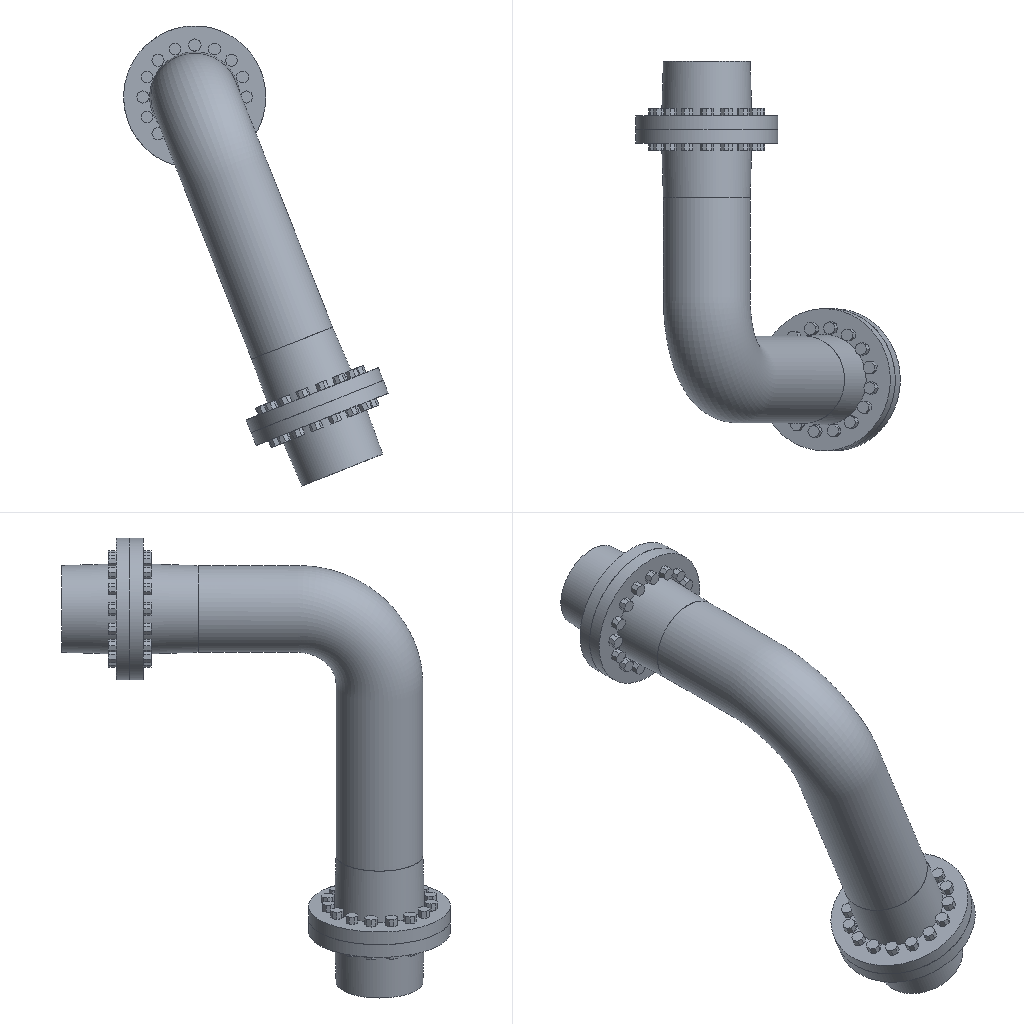Simulation study | abaqus
Set-up summary:
category,name,step,type,value,unit,region
solver,abaqus
solver,version,,,Abaqus/Explicit 2020
units,not stated in the deck,,not stated
analysis,deck,,transient,transient
load_step,Step-1,Step-1,transient
load_step,requested,,,1
mesh,nodes,,,69898
mesh,elements,,,46088
element_type,C3D8R,,solid,46088
load,load commands in deck,,count,4
bc,support commands in deck,,count,1
material,GUAN,,in results
material,SHUAN,,in results
check,setup vs results,,match,"per instance, exact: element labels, types and connectivity; labels of the nodes the elements use; coordinates of those nodes at SINGLE_PRECISION in 36 of 37 instance(s)"
Abaqus input file, long lists of numbers shortened, first 398 of 1239 lines:
*Heading
** Job name: Job-1 Model name: Model-1
** Generated by: Abaqus/CAE 2020
*Preprint, echo=NO, model=NO, history=NO, contact=NO
**
** PARTS
**
*Part, name=work-1
*Node
      1,   7.516,   71.639,    327.175
      2,   28.109,   71.639,   296.355
** (11603 more lines like these left out)
*Element, type=C3D8R
  1, 1914, 1854,  144,  143, 7833, 7773, 2131, 2140
  2, 1913, 1855, 1854, 1914, 7832, 7774, 7773, 7833
** (7830 more lines like these left out)
*Nset, nset=Set-2, generate
     1,  11605,      1
*Elset, elset=Set-2, generate
    1,  7832,     1
** Section: guan
*Solid Section, elset=Set-2, material=guan
,
*End Part
**
*Part, name=work-2
*Node
      1,   -133.467,  -53.341,   303.478
      2,   -129.716,  -53.341,   300.992
** (11398 more lines like these left out)
*Element, type=C3D8R
   1,   121,   122,   133,   162,     1,     2,    13,    42
   2,   162,   133,   134,   161,    42,    13,    14,    41
** (5638 more lines like these left out)
*Nset, nset=Set-2, generate
     1,  11400,      1
*Elset, elset=Set-2, generate
    1,  5640,     1
** Section: guan
*Solid Section, elset=Set-2, material=guan
,
*End Part
**
*Part, name=work-3
*Node
      1,   251.619,  -399.758,   -269.833
      2,   277.179,  -403.562,  -259.721
** (13338 more lines like these left out)
*Element, type=C3D8R
  1, 1985, 1926,  167,  166, 9413, 9354, 2193, 2202
  2, 1984, 1927, 1926, 1985, 9412, 9355, 9354, 9413
** (9574 more lines like these left out)
*Nset, nset=Set-2, generate
     1,  13340,      1
*Elset, elset=Set-2, generate
    1,  9576,     1
** Section: guan
*Solid Section, elset=Set-2, material=guan
,
*End Part
**
*Part, name=work-8
*Node
      1,  -77.419,   46.139,   165.583
      2,  -77.419,   46.139,   158.333
** (267 more lines like these left out)
*Element, type=C3D8R
 1, 130,  31, 123, 229,  29,   1,  30, 122
 2, 131,  32, 124, 228, 130,  31, 123, 229
** (174 more lines like these left out)
*Nset, nset=Set-1, generate
   1,  269,    1
*Elset, elset=Set-1, generate
   1,  176,    1
** Section: shuan
*Solid Section, elset=Set-1, material=shuan
,
*End Part
**
*Part, name=work-39
*Node
      1,    170.135,  -290.816,  -328.954
      2,   170.243,   -283.567,  -328.911
** (267 more lines like these left out)
*Element, type=C3D8R
 1, 130,  37, 123, 229,  29,   1,  30, 122
 2, 131,  36, 124, 228, 130,  37, 123, 229
** (174 more lines like these left out)
*Nset, nset=Set-1, generate
   1,  269,    1
*Elset, elset=Set-1, generate
   1,  176,    1
** Section: shuan
*Solid Section, elset=Set-1, material=shuan
,
*End Part
**
**
** ASSEMBLY
**
*Assembly, name=Assembly
**
*Instance, name=work-1-1, part=work-1
*End Instance
**
*Instance, name=work-2-1, part=work-2
*End Instance
**
*Instance, name=work-3-1, part=work-3
*End Instance
**
*Instance, name=work-8-1, part=work-8
   10.51,     0.5,    -0.5831
*End Instance
**
*Instance, name=work-39-1, part=work-39
   10.692,    -0.1838,     4.23
*End Instance
**
*Instance, name=work-1-2, part=work-1
 -133.819,   143.277,           0.
 -133.819,   143.277,           0.,  -133.819,   143.277,           1.,         180.
*End Instance
**
*Instance, name=work-3-2, part=work-3
156.459, -747.905, -676.855
156.459, -747.905, -676.855, 157.38, -748.043, -676.49,         180.
*End Instance
**
*Instance, name=work-39-1-rad-2, part=work-39
-124.956, -37.925, -49.433
-124.956, -37.925, -49.433, -125.324, -37.925, -48.504, 22.5
*End Instance
**
*Instance, name=work-39-1-rad-3, part=work-39
-236.848, -128.617, -93.699
-236.848, -128.617, -93.699, -237.216, -128.617, -92.769, 45.
*End Instance
**
*Instance, name=work-39-1-rad-4, part=work-39
-307.95, -258.454, -121.827
-307.95, -258.454, -121.827, -308.318, -258.454, -120.898, 67.5
*End Instance
**
*Instance, name=work-39-1-rad-5, part=work-39
-327.438, -407.67, -129.537
-327.438, -407.67, -129.537, -327.806, -407.67, -128.607, 90.
*End Instance
**
*Instance, name=work-39-1-rad-6, part=work-39
-292.343, -553.547, -115.653
-292.343, -553.547, -115.653, -292.711, -553.547, -114.723, 112.5
*End Instance
**
*Instance, name=work-39-1-rad-7, part=work-39
-208.01, -673.877, -82.29
-208.01, -673.877, -82.29, -208.378, -673.877, -81.361, 135.
*End Instance
**
*Instance, name=work-39-1-rad-8, part=work-39
-87.277, -750.341, -34.528
-87.277, -750.341, -34.528, -87.645, -750.341, -33.598, 157.5
*End Instance
**
*Instance, name=work-39-1-rad-9, part=work-39
51.475,  -771.298, 20.364
51.475,  -771.298, 20.364, 51.107,  -771.298, 21.294,         180.
*End Instance
**
*Instance, name=work-39-1-rad-10, part=work-39
187.123, -733.558, 74.027
187.123, -733.558, 74.027, 186.755, -733.558, 74.957, 202.5
*End Instance
**
*Instance, name=work-39-1-rad-11, part=work-39
299.015, -642.865, 118.293
299.015, -642.865, 118.293, 298.647, -642.865, 119.223, 225.
*End Instance
**
*Instance, name=work-39-1-rad-12, part=work-39
370.118, -513.028, 146.421
370.118, -513.028, 146.421, 370.485, -513.028, 145.491, 112.5
*End Instance
**
*Instance, name=work-39-1-rad-13, part=work-39
389.605, -363.812, 154.131
389.605, -363.812, 154.131, 389.973, -363.812, 153.201, 90.
*End Instance
**
*Instance, name=work-39-1-rad-14, part=work-39
354.511, -217.935, 140.247
354.511, -217.935, 140.247, 354.879, -217.935, 139.317, 67.5
*End Instance
**
*Instance, name=work-39-1-rad-15, part=work-39
270.178, -97.605, 106.884
270.178, -97.605, 106.884, 270.545, -97.605, 105.954, 45.
*End Instance
**
*Instance, name=work-39-1-rad-16, part=work-39
149.445, -21.141, 59.121
149.445, -21.141, 59.121, 149.812, -21.141, 58.192, 22.5
*End Instance
**
*Instance, name=work-8-1-rad-2, part=work-8
104.338,     0.5, 48.88
104.338,     0.5, 48.88, 104.338, -0.5, 48.88, 22.5
*End Instance
**
*Instance, name=work-8-1-rad-3, part=work-8
172.094,     0.5, 130.484
172.094,     0.5, 130.484, 172.094, -0.5, 130.484, 45.
*End Instance
**
*Instance, name=work-8-1-rad-4, part=work-8
203.465,     0.5, 231.805
203.465,     0.5, 231.805, 203.465, -0.5, 231.805, 67.5
*End Instance
**
*Instance, name=work-8-1-rad-5, part=work-8
  193.674,     0.5,   337.419
  193.674,     0.5,   337.419,   193.674, -0.5,   337.419, 90.
*End Instance
**
*Instance, name=work-8-1-rad-6, part=work-8
144.211,     0.5, 431.247
144.211,     0.5, 431.247, 144.211, -0.5, 431.247, 112.5
*End Instance
**
*Instance, name=work-8-1-rad-7, part=work-8
62.607,     0.5, 499.004
62.607,     0.5, 499.004, 62.607, 1.5, 499.004, 225.
*End Instance
**
*Instance, name=work-8-1-rad-8, part=work-8
-38.715,     0.5, 530.374
-38.715,     0.5, 530.374, -38.715, 1.5, 530.374, 202.5
*End Instance
**
*Instance, name=work-8-1-rad-9, part=work-8
 -144.329,     0.5,   520.583
 -144.329,     0.5,   520.583,  -144.329,     1.5,   520.583,         180.
*End Instance
**
*Instance, name=work-8-1-rad-10, part=work-8
-238.156,     0.5, 471.12
-238.156,     0.5, 471.12, -238.156, 1.5, 471.12, 157.5
*End Instance
**
*Instance, name=work-8-1-rad-11, part=work-8
-305.913,     0.5, 389.516
-305.913,     0.5, 389.516, -305.913, 1.5, 389.516, 135.
*End Instance
**
*Instance, name=work-8-1-rad-12, part=work-8
-337.284,     0.5, 288.195
-337.284,     0.5, 288.195, -337.284, 1.5, 288.195, 112.5
*End Instance
**
*Instance, name=work-8-1-rad-13, part=work-8
 -327.493,     0.5,   182.581
 -327.493,     0.5,   182.581,  -327.493, 1.5,   182.581, 90.
*End Instance
**
*Instance, name=work-8-1-rad-14, part=work-8
-278.03,     0.5, 88.753
-278.03,     0.5, 88.753, -278.03, 1.5, 88.753, 67.5
*End Instance
**
*Instance, name=work-8-1-rad-15, part=work-8
-196.426,     0.5, 20.996
-196.426,     0.5, 20.996, -196.426, 1.5, 20.996, 45.
*End Instance
**
*Instance, name=work-8-1-rad-16, part=work-8
-95.104,     0.5, -10.374
-95.104,     0.5, -10.374, -95.104, 1.5, -10.374, 22.5
*End Instance
**
*Nset, nset=Set-1, instance=work-1-1, generate
     1,  11605,      1
*Nset, nset=Set-1, instance=work-2-1, generate
     1,  11400,      1
*Nset, nset=Set-1, instance=work-3-1, generate
     1,  13340,      1
*Nset, nset=Set-1, instance=work-39-1-rad-2, generate
   1,  269,    1
*Nset, nset=Set-1, instance=work-39-1-rad-10, generate
   1,  269,    1
*Nset, nset=Set-1, instance=work-39-1-rad-6, generate
   1,  269,    1
*Nset, nset=Set-1, instance=work-39-1-rad-14, generate
   1,  269,    1
*Nset, nset=Set-1, instance=work-1-2, generate
     1,  11605,      1
*Nset, nset=Set-1, instance=work-39-1-rad-4, generate
   1,  269,    1
*Nset, nset=Set-1, instance=work-39-1-rad-12, generate
   1,  269,    1
*Nset, nset=Set-1, instance=work-39-1-rad-8, generate
   1,  269,    1
*Nset, nset=Set-1, instance=work-39-1-rad-16, generate
   1,  269,    1
*Nset, nset=Set-1, instance=work-8-1, generate
   1,  269,    1
*Nset, nset=Set-1, instance=work-39-1, generate
   1,  269,    1
*Nset, nset=Set-1, instance=work-39-1-rad-3, generate
   1,  269,    1
*Nset, nset=Set-1, instance=work-39-1-rad-11, generate
   1,  269,    1
*Nset, nset=Set-1, instance=work-3-2, generate
     1,  13340,      1
*Nset, nset=Set-1, instance=work-39-1-rad-7, generate
   1,  269,    1
*Nset, nset=Set-1, instance=work-39-1-rad-15, generate
   1,  269,    1
*Nset, nset=Set-1, instance=work-39-1-rad-5, generate
   1,  269,    1
*Nset, nset=Set-1, instance=work-39-1-rad-13, generate
   1,  269,    1
*Nset, nset=Set-1, instance=work-39-1-rad-9, generate
   1,  269,    1
*Nset, nset=Set-1, instance=work-8-1-rad-2, generate
   1,  269,    1
*Nset, nset=Set-1, instance=work-8-1-rad-4, generate
   1,  269,    1
*Nset, nset=Set-1, instance=work-8-1-rad-6, generate
   1,  269,    1
*Nset, nset=Set-1, instance=work-8-1-rad-10, generate
   1,  269,    1
*Nset, nset=Set-1, instance=work-8-1-rad-14, generate
   1,  269,    1
*Nset, nset=Set-1, instance=work-8-1-rad-8, generate
   1,  269,    1
*Nset, nset=Set-1, instance=work-8-1-rad-12, generate
   1,  269,    1
*Nset, nset=Set-1, instance=work-8-1-rad-16, generate
   1,  269,    1
*Nset, nset=Set-1, instance=work-8-1-rad-3, generate
   1,  269,    1
*Nset, nset=Set-1, instance=work-8-1-rad-7, generate
   1,  269,    1
*Nset, nset=Set-1, instance=work-8-1-rad-11, generate
   1,  269,    1
*Nset, nset=Set-1, instance=work-8-1-rad-15, generate
   1,  269,    1
*Nset, nset=Set-1, instance=work-8-1-rad-5, generate
   1,  269,    1
*Nset, nset=Set-1, instance=work-8-1-rad-13, generate
   1,  269,    1
*Nset, nset=Set-1, instance=work-8-1-rad-9, generate
   1,  269,    1
*Elset, elset=Set-1, instance=work-1-1, generate
    1,  7832,     1
*Elset, elset=Set-1, instance=work-2-1, generate
    1,  5640,     1
*Elset, elset=Set-1, instance=work-3-1, generate
    1,  9576,     1
*Elset, elset=Set-1, instance=work-39-1-rad-2, generate
   1,  176,    1
*Elset, elset=Set-1, instance=work-39-1-rad-10, generate
   1,  176,    1
*Elset, elset=Set-1, instance=work-39-1-rad-6, generate
   1,  176,    1
*Elset, elset=Set-1, instance=work-39-1-rad-14, generate
   1,  176,    1
*Elset, elset=Set-1, instance=work-1-2, generate
    1,  7832,     1
*Elset, elset=Set-1, instance=work-39-1-rad-4, generate
   1,  176,    1
*Elset, elset=Set-1, instance=work-39-1-rad-12, generate
   1,  176,    1
*Elset, elset=Set-1, instance=work-39-1-rad-8, generate
   1,  176,    1
*Elset, elset=Set-1, instance=work-39-1-rad-16, generate
   1,  176,    1
*Elset, elset=Set-1, instance=work-8-1, generate
   1,  176,    1
*Elset, elset=Set-1, instance=work-39-1, generate
   1,  176,    1
*Elset, elset=Set-1, instance=work-39-1-rad-3, generate
   1,  176,    1
*Elset, elset=Set-1, instance=work-39-1-rad-11, generate
   1,  176,    1
*Elset, elset=Set-1, instance=work-3-2, generate
    1,  9576,     1
*Elset, elset=Set-1, instance=work-39-1-rad-7, generate
   1,  176,    1
*Elset, elset=Set-1, instance=work-39-1-rad-15, generate
   1,  176,    1
*Elset, elset=Set-1, instance=work-39-1-rad-5, generate
   1,  176,    1
*Elset, elset=Set-1, instance=work-39-1-rad-13, generate
   1,  176,    1
*Elset, elset=Set-1, instance=work-39-1-rad-9, generate
   1,  176,    1
*Elset, elset=Set-1, instance=work-8-1-rad-2, generate
Last 584 lines:
** (233 more lines like these left out)
*Elset, elset=_Surf-17_S5, internal, instance=work-3-1, generate
 7729,  9576,     1
*Surface, type=ELEMENT, name=Surf-17
_Surf-17_S3, S3
_Surf-17_S6, S6
_Surf-17_S4, S4
_Surf-17_S5, S5
*Elset, elset=_Surf-18_S4, internal, instance=work-2-1
    1,    2,    3,    4,    5,    6,    7,    8,    9,   10,   11,   12,   13,   14,   15,   16
   23,   24,   25,   26,   27,   28,   29,   30,   31,   32,   33,   34,   35,   36,   37,   38
** (233 more lines like these left out)
*Elset, elset=_Surf-18_S6, internal, instance=work-2-1
   17,   18,   19,   20,   21,   22,   47,   48,   49,   50,   51,   52,   53,   54,   55,   56
   57,   58,   59,   60,   77,   78,   79,   80,   81,   82,  107,  108,  109,  110,  111,  112
** (116 more lines like these left out)
*Surface, type=ELEMENT, name=Surf-18
_Surf-18_S4, S4
_Surf-18_S6, S6
*Elset, elset=_m_Surf-5_S4, internal, instance=work-1-1
 4244, 4264, 4285, 4305, 4326, 4346, 4367, 4387, 4408, 4428, 4449, 4469, 4490, 4510, 4531, 4551
 4572, 4592, 4613, 4633, 4654, 4674, 4695, 4715, 4736, 4756, 4777, 4797, 4818, 4838, 4859, 4879
** (9 more lines like these left out)
*Elset, elset=_m_Surf-5_S4, internal, instance=work-3-1, generate
 7749,  9576,    21
*Surface, type=ELEMENT, name=m_Surf-5
_m_Surf-5_S4, S4
*Elset, elset=_m_Surf-7_S1, internal, instance=work-1-2
    1,    2,    3,    4,    5,    6,    7,    8,    9,   10,   11,   12,   13,   14,   15,   16
   17,   18,   19,   20,   21,   22,   23,   24,   25,   26,   27,   28,   29,   30,   31,   32
** (60 more lines like these left out)
*Surface, type=ELEMENT, name=m_Surf-7
_m_Surf-7_S1, S1
*Elset, elset=_m_Surf-9_S5, internal, instance=work-1-2, generate
 4265,  7832,    41
*Elset, elset=_m_Surf-9_S1, internal, instance=work-1-2
    1,    2,    3,    4,    5,    6,    7,    8,    9,   10,   11,   12,   13,   14,   15,   16
   17,   18,   19,   20,   21,   22,   23,   24,   25,   26,   27,   28,   29,   30,   31,   32
** (60 more lines like these left out)
*Surface, type=ELEMENT, name=m_Surf-9
_m_Surf-9_S5, S5
_m_Surf-9_S1, S1
*Elset, elset=_m_Surf-10_S3, internal, instance=work-3-2, generate
 2999,  6740,    43
*Elset, elset=_m_Surf-10_S6, internal, instance=work-3-2, generate
 7729,  9556,    21
*Elset, elset=_m_Surf-10_S1, internal, instance=work-3-2
    1,    2,    3,    4,    5,    6,    7,    8,    9,   10,   11,   12,   13,   14,   15,   16
   17,   18,   19,   20,   21,   22,   23,   24,   25,   26,   27,   28,   29,   30,   31,   32
** (60 more lines like these left out)
*Surface, type=ELEMENT, name=m_Surf-10
_m_Surf-10_S3, S3
_m_Surf-10_S6, S6
_m_Surf-10_S1, S1
*Elset, elset=_m_Surf-12_S5, internal, instance=work-1-2, generate
 4265,  7832,    41
*Elset, elset=_m_Surf-12_S1, internal, instance=work-1-2
    1,    2,    3,    4,    5,    6,    7,    8,    9,   10,   11,   12,   13,   14,   15,   16
   17,   18,   19,   20,   21,   22,   23,   24,   25,   26,   27,   28,   29,   30,   31,   32
** (60 more lines like these left out)
*Surface, type=ELEMENT, name=m_Surf-12
_m_Surf-12_S5, S5
_m_Surf-12_S1, S1
*Elset, elset=_m_Surf-13_S1, internal, instance=work-8-1
  97,  98, 107, 108, 117, 118, 130, 131, 137, 138, 147, 148, 157, 158, 167, 168
*Elset, elset=_m_Surf-13_S1, internal, instance=work-8-1-rad-2
  97,  98, 107, 108, 117, 118, 130, 131, 137, 138, 147, 148, 157, 158, 167, 168
*Elset, elset=_m_Surf-13_S1, internal, instance=work-8-1-rad-4
  97,  98, 107, 108, 117, 118, 130, 131, 137, 138, 147, 148, 157, 158, 167, 168
*Elset, elset=_m_Surf-13_S1, internal, instance=work-8-1-rad-6
  97,  98, 107, 108, 117, 118, 130, 131, 137, 138, 147, 148, 157, 158, 167, 168
*Elset, elset=_m_Surf-13_S1, internal, instance=work-8-1-rad-10
  97,  98, 107, 108, 117, 118, 130, 131, 137, 138, 147, 148, 157, 158, 167, 168
*Elset, elset=_m_Surf-13_S1, internal, instance=work-8-1-rad-14
  97,  98, 107, 108, 117, 118, 130, 131, 137, 138, 147, 148, 157, 158, 167, 168
*Elset, elset=_m_Surf-13_S1, internal, instance=work-8-1-rad-8
  97,  98, 107, 108, 117, 118, 130, 131, 137, 138, 147, 148, 157, 158, 167, 168
*Elset, elset=_m_Surf-13_S1, internal, instance=work-8-1-rad-12
  97,  98, 107, 108, 117, 118, 130, 131, 137, 138, 147, 148, 157, 158, 167, 168
*Elset, elset=_m_Surf-13_S1, internal, instance=work-8-1-rad-16
  97,  98, 107, 108, 117, 118, 130, 131, 137, 138, 147, 148, 157, 158, 167, 168
*Elset, elset=_m_Surf-13_S1, internal, instance=work-8-1-rad-3
  97,  98, 107, 108, 117, 118, 130, 131, 137, 138, 147, 148, 157, 158, 167, 168
*Elset, elset=_m_Surf-13_S1, internal, instance=work-8-1-rad-7
  97,  98, 107, 108, 117, 118, 130, 131, 137, 138, 147, 148, 157, 158, 167, 168
*Elset, elset=_m_Surf-13_S1, internal, instance=work-8-1-rad-11
  97,  98, 107, 108, 117, 118, 130, 131, 137, 138, 147, 148, 157, 158, 167, 168
*Elset, elset=_m_Surf-13_S1, internal, instance=work-8-1-rad-15
  97,  98, 107, 108, 117, 118, 130, 131, 137, 138, 147, 148, 157, 158, 167, 168
*Elset, elset=_m_Surf-13_S1, internal, instance=work-8-1-rad-5
  97,  98, 107, 108, 117, 118, 130, 131, 137, 138, 147, 148, 157, 158, 167, 168
*Elset, elset=_m_Surf-13_S1, internal, instance=work-8-1-rad-13
  97,  98, 107, 108, 117, 118, 130, 131, 137, 138, 147, 148, 157, 158, 167, 168
*Elset, elset=_m_Surf-13_S1, internal, instance=work-8-1-rad-9
  97,  98, 107, 108, 117, 118, 130, 131, 137, 138, 147, 148, 157, 158, 167, 168
*Elset, elset=_m_Surf-13_S3, internal, instance=work-8-1
  5,  6,  7,  8, 17, 18, 19, 20, 25, 26, 27, 28, 49, 50, 51, 52
 73, 74, 75, 76, 89, 90, 91, 92, 93, 94, 95, 96
*Elset, elset=_m_Surf-13_S3, internal, instance=work-8-1-rad-2
  5,  6,  7,  8, 17, 18, 19, 20, 25, 26, 27, 28, 49, 50, 51, 52
 73, 74, 75, 76, 89, 90, 91, 92, 93, 94, 95, 96
*Elset, elset=_m_Surf-13_S3, internal, instance=work-8-1-rad-4
  5,  6,  7,  8, 17, 18, 19, 20, 25, 26, 27, 28, 49, 50, 51, 52
 73, 74, 75, 76, 89, 90, 91, 92, 93, 94, 95, 96
*Elset, elset=_m_Surf-13_S3, internal, instance=work-8-1-rad-6
  5,  6,  7,  8, 17, 18, 19, 20, 25, 26, 27, 28, 49, 50, 51, 52
 73, 74, 75, 76, 89, 90, 91, 92, 93, 94, 95, 96
*Elset, elset=_m_Surf-13_S3, internal, instance=work-8-1-rad-10
  5,  6,  7,  8, 17, 18, 19, 20, 25, 26, 27, 28, 49, 50, 51, 52
 73, 74, 75, 76, 89, 90, 91, 92, 93, 94, 95, 96
*Elset, elset=_m_Surf-13_S3, internal, instance=work-8-1-rad-14
  5,  6,  7,  8, 17, 18, 19, 20, 25, 26, 27, 28, 49, 50, 51, 52
 73, 74, 75, 76, 89, 90, 91, 92, 93, 94, 95, 96
*Elset, elset=_m_Surf-13_S3, internal, instance=work-8-1-rad-8
  5,  6,  7,  8, 17, 18, 19, 20, 25, 26, 27, 28, 49, 50, 51, 52
 73, 74, 75, 76, 89, 90, 91, 92, 93, 94, 95, 96
*Elset, elset=_m_Surf-13_S3, internal, instance=work-8-1-rad-12
  5,  6,  7,  8, 17, 18, 19, 20, 25, 26, 27, 28, 49, 50, 51, 52
 73, 74, 75, 76, 89, 90, 91, 92, 93, 94, 95, 96
*Elset, elset=_m_Surf-13_S3, internal, instance=work-8-1-rad-16
  5,  6,  7,  8, 17, 18, 19, 20, 25, 26, 27, 28, 49, 50, 51, 52
 73, 74, 75, 76, 89, 90, 91, 92, 93, 94, 95, 96
*Elset, elset=_m_Surf-13_S3, internal, instance=work-8-1-rad-3
  5,  6,  7,  8, 17, 18, 19, 20, 25, 26, 27, 28, 49, 50, 51, 52
 73, 74, 75, 76, 89, 90, 91, 92, 93, 94, 95, 96
*Elset, elset=_m_Surf-13_S3, internal, instance=work-8-1-rad-7
  5,  6,  7,  8, 17, 18, 19, 20, 25, 26, 27, 28, 49, 50, 51, 52
 73, 74, 75, 76, 89, 90, 91, 92, 93, 94, 95, 96
*Elset, elset=_m_Surf-13_S3, internal, instance=work-8-1-rad-11
  5,  6,  7,  8, 17, 18, 19, 20, 25, 26, 27, 28, 49, 50, 51, 52
 73, 74, 75, 76, 89, 90, 91, 92, 93, 94, 95, 96
*Elset, elset=_m_Surf-13_S3, internal, instance=work-8-1-rad-15
  5,  6,  7,  8, 17, 18, 19, 20, 25, 26, 27, 28, 49, 50, 51, 52
 73, 74, 75, 76, 89, 90, 91, 92, 93, 94, 95, 96
*Elset, elset=_m_Surf-13_S3, internal, instance=work-8-1-rad-5
  5,  6,  7,  8, 17, 18, 19, 20, 25, 26, 27, 28, 49, 50, 51, 52
 73, 74, 75, 76, 89, 90, 91, 92, 93, 94, 95, 96
*Elset, elset=_m_Surf-13_S3, internal, instance=work-8-1-rad-13
  5,  6,  7,  8, 17, 18, 19, 20, 25, 26, 27, 28, 49, 50, 51, 52
 73, 74, 75, 76, 89, 90, 91, 92, 93, 94, 95, 96
*Elset, elset=_m_Surf-13_S3, internal, instance=work-8-1-rad-9
  5,  6,  7,  8, 17, 18, 19, 20, 25, 26, 27, 28, 49, 50, 51, 52
 73, 74, 75, 76, 89, 90, 91, 92, 93, 94, 95, 96
*Elset, elset=_m_Surf-13_S4, internal, instance=work-8-1
  9, 10, 11, 12, 21, 22, 23, 24, 29, 30, 31, 32, 53, 54, 55, 56
 81, 82, 83, 84
*Elset, elset=_m_Surf-13_S4, internal, instance=work-8-1-rad-2
  9, 10, 11, 12, 21, 22, 23, 24, 29, 30, 31, 32, 53, 54, 55, 56
 81, 82, 83, 84
*Elset, elset=_m_Surf-13_S4, internal, instance=work-8-1-rad-4
  9, 10, 11, 12, 21, 22, 23, 24, 29, 30, 31, 32, 53, 54, 55, 56
 81, 82, 83, 84
*Elset, elset=_m_Surf-13_S4, internal, instance=work-8-1-rad-6
  9, 10, 11, 12, 21, 22, 23, 24, 29, 30, 31, 32, 53, 54, 55, 56
 81, 82, 83, 84
*Elset, elset=_m_Surf-13_S4, internal, instance=work-8-1-rad-10
  9, 10, 11, 12, 21, 22, 23, 24, 29, 30, 31, 32, 53, 54, 55, 56
 81, 82, 83, 84
*Elset, elset=_m_Surf-13_S4, internal, instance=work-8-1-rad-14
  9, 10, 11, 12, 21, 22, 23, 24, 29, 30, 31, 32, 53, 54, 55, 56
 81, 82, 83, 84
*Elset, elset=_m_Surf-13_S4, internal, instance=work-8-1-rad-8
  9, 10, 11, 12, 21, 22, 23, 24, 29, 30, 31, 32, 53, 54, 55, 56
 81, 82, 83, 84
*Elset, elset=_m_Surf-13_S4, internal, instance=work-8-1-rad-12
  9, 10, 11, 12, 21, 22, 23, 24, 29, 30, 31, 32, 53, 54, 55, 56
 81, 82, 83, 84
*Elset, elset=_m_Surf-13_S4, internal, instance=work-8-1-rad-16
  9, 10, 11, 12, 21, 22, 23, 24, 29, 30, 31, 32, 53, 54, 55, 56
 81, 82, 83, 84
*Elset, elset=_m_Surf-13_S4, internal, instance=work-8-1-rad-3
  9, 10, 11, 12, 21, 22, 23, 24, 29, 30, 31, 32, 53, 54, 55, 56
 81, 82, 83, 84
*Elset, elset=_m_Surf-13_S4, internal, instance=work-8-1-rad-7
  9, 10, 11, 12, 21, 22, 23, 24, 29, 30, 31, 32, 53, 54, 55, 56
 81, 82, 83, 84
*Elset, elset=_m_Surf-13_S4, internal, instance=work-8-1-rad-11
  9, 10, 11, 12, 21, 22, 23, 24, 29, 30, 31, 32, 53, 54, 55, 56
 81, 82, 83, 84
*Elset, elset=_m_Surf-13_S4, internal, instance=work-8-1-rad-15
  9, 10, 11, 12, 21, 22, 23, 24, 29, 30, 31, 32, 53, 54, 55, 56
 81, 82, 83, 84
*Elset, elset=_m_Surf-13_S4, internal, instance=work-8-1-rad-5
  9, 10, 11, 12, 21, 22, 23, 24, 29, 30, 31, 32, 53, 54, 55, 56
 81, 82, 83, 84
*Elset, elset=_m_Surf-13_S4, internal, instance=work-8-1-rad-13
  9, 10, 11, 12, 21, 22, 23, 24, 29, 30, 31, 32, 53, 54, 55, 56
 81, 82, 83, 84
*Elset, elset=_m_Surf-13_S4, internal, instance=work-8-1-rad-9
  9, 10, 11, 12, 21, 22, 23, 24, 29, 30, 31, 32, 53, 54, 55, 56
 81, 82, 83, 84
*Elset, elset=_m_Surf-13_S2, internal, instance=work-8-1
 37, 38, 39, 40, 41, 42, 43, 44, 61, 62, 63, 64, 65, 66, 67, 68
*Elset, elset=_m_Surf-13_S2, internal, instance=work-8-1-rad-2
 37, 38, 39, 40, 41, 42, 43, 44, 61, 62, 63, 64, 65, 66, 67, 68
*Elset, elset=_m_Surf-13_S2, internal, instance=work-8-1-rad-4
 37, 38, 39, 40, 41, 42, 43, 44, 61, 62, 63, 64, 65, 66, 67, 68
*Elset, elset=_m_Surf-13_S2, internal, instance=work-8-1-rad-6
 37, 38, 39, 40, 41, 42, 43, 44, 61, 62, 63, 64, 65, 66, 67, 68
*Elset, elset=_m_Surf-13_S2, internal, instance=work-8-1-rad-10
 37, 38, 39, 40, 41, 42, 43, 44, 61, 62, 63, 64, 65, 66, 67, 68
*Elset, elset=_m_Surf-13_S2, internal, instance=work-8-1-rad-14
 37, 38, 39, 40, 41, 42, 43, 44, 61, 62, 63, 64, 65, 66, 67, 68
*Elset, elset=_m_Surf-13_S2, internal, instance=work-8-1-rad-8
 37, 38, 39, 40, 41, 42, 43, 44, 61, 62, 63, 64, 65, 66, 67, 68
*Elset, elset=_m_Surf-13_S2, internal, instance=work-8-1-rad-12
 37, 38, 39, 40, 41, 42, 43, 44, 61, 62, 63, 64, 65, 66, 67, 68
*Elset, elset=_m_Surf-13_S2, internal, instance=work-8-1-rad-16
 37, 38, 39, 40, 41, 42, 43, 44, 61, 62, 63, 64, 65, 66, 67, 68
*Elset, elset=_m_Surf-13_S2, internal, instance=work-8-1-rad-3
 37, 38, 39, 40, 41, 42, 43, 44, 61, 62, 63, 64, 65, 66, 67, 68
*Elset, elset=_m_Surf-13_S2, internal, instance=work-8-1-rad-7
 37, 38, 39, 40, 41, 42, 43, 44, 61, 62, 63, 64, 65, 66, 67, 68
*Elset, elset=_m_Surf-13_S2, internal, instance=work-8-1-rad-11
 37, 38, 39, 40, 41, 42, 43, 44, 61, 62, 63, 64, 65, 66, 67, 68
*Elset, elset=_m_Surf-13_S2, internal, instance=work-8-1-rad-15
 37, 38, 39, 40, 41, 42, 43, 44, 61, 62, 63, 64, 65, 66, 67, 68
*Elset, elset=_m_Surf-13_S2, internal, instance=work-8-1-rad-5
 37, 38, 39, 40, 41, 42, 43, 44, 61, 62, 63, 64, 65, 66, 67, 68
*Elset, elset=_m_Surf-13_S2, internal, instance=work-8-1-rad-13
 37, 38, 39, 40, 41, 42, 43, 44, 61, 62, 63, 64, 65, 66, 67, 68
*Elset, elset=_m_Surf-13_S2, internal, instance=work-8-1-rad-9
 37, 38, 39, 40, 41, 42, 43, 44, 61, 62, 63, 64, 65, 66, 67, 68
*Surface, type=ELEMENT, name=m_Surf-13
_m_Surf-13_S1, S1
_m_Surf-13_S3, S3
_m_Surf-13_S4, S4
_m_Surf-13_S2, S2
*Elset, elset=_m_Surf-15_S1, internal, instance=work-39-1
  97,  98, 107, 108, 117, 118, 127, 128, 140, 141, 147, 148, 160, 161, 167, 168
*Elset, elset=_m_Surf-15_S1, internal, instance=work-39-1-rad-2
  97,  98, 107, 108, 117, 118, 127, 128, 140, 141, 147, 148, 160, 161, 167, 168
*Elset, elset=_m_Surf-15_S1, internal, instance=work-39-1-rad-4
  97,  98, 107, 108, 117, 118, 127, 128, 140, 141, 147, 148, 160, 161, 167, 168
*Elset, elset=_m_Surf-15_S1, internal, instance=work-39-1-rad-6
  97,  98, 107, 108, 117, 118, 127, 128, 140, 141, 147, 148, 160, 161, 167, 168
*Elset, elset=_m_Surf-15_S1, internal, instance=work-39-1-rad-10
  97,  98, 107, 108, 117, 118, 127, 128, 140, 141, 147, 148, 160, 161, 167, 168
*Elset, elset=_m_Surf-15_S1, internal, instance=work-39-1-rad-14
  97,  98, 107, 108, 117, 118, 127, 128, 140, 141, 147, 148, 160, 161, 167, 168
*Elset, elset=_m_Surf-15_S1, internal, instance=work-39-1-rad-8
  97,  98, 107, 108, 117, 118, 127, 128, 140, 141, 147, 148, 160, 161, 167, 168
*Elset, elset=_m_Surf-15_S1, internal, instance=work-39-1-rad-12
  97,  98, 107, 108, 117, 118, 127, 128, 140, 141, 147, 148, 160, 161, 167, 168
*Elset, elset=_m_Surf-15_S1, internal, instance=work-39-1-rad-16
  97,  98, 107, 108, 117, 118, 127, 128, 140, 141, 147, 148, 160, 161, 167, 168
*Elset, elset=_m_Surf-15_S1, internal, instance=work-39-1-rad-3
  97,  98, 107, 108, 117, 118, 127, 128, 140, 141, 147, 148, 160, 161, 167, 168
*Elset, elset=_m_Surf-15_S1, internal, instance=work-39-1-rad-7
  97,  98, 107, 108, 117, 118, 127, 128, 140, 141, 147, 148, 160, 161, 167, 168
*Elset, elset=_m_Surf-15_S1, internal, instance=work-39-1-rad-11
  97,  98, 107, 108, 117, 118, 127, 128, 140, 141, 147, 148, 160, 161, 167, 168
*Elset, elset=_m_Surf-15_S1, internal, instance=work-39-1-rad-15
  97,  98, 107, 108, 117, 118, 127, 128, 140, 141, 147, 148, 160, 161, 167, 168
*Elset, elset=_m_Surf-15_S1, internal, instance=work-39-1-rad-5
  97,  98, 107, 108, 117, 118, 127, 128, 140, 141, 147, 148, 160, 161, 167, 168
*Elset, elset=_m_Surf-15_S1, internal, instance=work-39-1-rad-13
  97,  98, 107, 108, 117, 118, 127, 128, 140, 141, 147, 148, 160, 161, 167, 168
*Elset, elset=_m_Surf-15_S1, internal, instance=work-39-1-rad-9
  97,  98, 107, 108, 117, 118, 127, 128, 140, 141, 147, 148, 160, 161, 167, 168
*Elset, elset=_m_Surf-15_S3, internal, instance=work-39-1
  5,  6,  7,  8, 17, 18, 19, 20, 25, 26, 27, 28, 49, 50, 51, 52
 77, 78, 79, 80, 89, 90, 91, 92, 93, 94, 95, 96
*Elset, elset=_m_Surf-15_S3, internal, instance=work-39-1-rad-2
  5,  6,  7,  8, 17, 18, 19, 20, 25, 26, 27, 28, 49, 50, 51, 52
 77, 78, 79, 80, 89, 90, 91, 92, 93, 94, 95, 96
*Elset, elset=_m_Surf-15_S3, internal, instance=work-39-1-rad-4
  5,  6,  7,  8, 17, 18, 19, 20, 25, 26, 27, 28, 49, 50, 51, 52
 77, 78, 79, 80, 89, 90, 91, 92, 93, 94, 95, 96
*Elset, elset=_m_Surf-15_S3, internal, instance=work-39-1-rad-6
  5,  6,  7,  8, 17, 18, 19, 20, 25, 26, 27, 28, 49, 50, 51, 52
 77, 78, 79, 80, 89, 90, 91, 92, 93, 94, 95, 96
*Elset, elset=_m_Surf-15_S3, internal, instance=work-39-1-rad-10
  5,  6,  7,  8, 17, 18, 19, 20, 25, 26, 27, 28, 49, 50, 51, 52
 77, 78, 79, 80, 89, 90, 91, 92, 93, 94, 95, 96
*Elset, elset=_m_Surf-15_S3, internal, instance=work-39-1-rad-14
  5,  6,  7,  8, 17, 18, 19, 20, 25, 26, 27, 28, 49, 50, 51, 52
 77, 78, 79, 80, 89, 90, 91, 92, 93, 94, 95, 96
*Elset, elset=_m_Surf-15_S3, internal, instance=work-39-1-rad-8
  5,  6,  7,  8, 17, 18, 19, 20, 25, 26, 27, 28, 49, 50, 51, 52
 77, 78, 79, 80, 89, 90, 91, 92, 93, 94, 95, 96
*Elset, elset=_m_Surf-15_S3, internal, instance=work-39-1-rad-12
  5,  6,  7,  8, 17, 18, 19, 20, 25, 26, 27, 28, 49, 50, 51, 52
 77, 78, 79, 80, 89, 90, 91, 92, 93, 94, 95, 96
*Elset, elset=_m_Surf-15_S3, internal, instance=work-39-1-rad-16
  5,  6,  7,  8, 17, 18, 19, 20, 25, 26, 27, 28, 49, 50, 51, 52
 77, 78, 79, 80, 89, 90, 91, 92, 93, 94, 95, 96
*Elset, elset=_m_Surf-15_S3, internal, instance=work-39-1-rad-3
  5,  6,  7,  8, 17, 18, 19, 20, 25, 26, 27, 28, 49, 50, 51, 52
 77, 78, 79, 80, 89, 90, 91, 92, 93, 94, 95, 96
*Elset, elset=_m_Surf-15_S3, internal, instance=work-39-1-rad-7
  5,  6,  7,  8, 17, 18, 19, 20, 25, 26, 27, 28, 49, 50, 51, 52
 77, 78, 79, 80, 89, 90, 91, 92, 93, 94, 95, 96
*Elset, elset=_m_Surf-15_S3, internal, instance=work-39-1-rad-11
  5,  6,  7,  8, 17, 18, 19, 20, 25, 26, 27, 28, 49, 50, 51, 52
 77, 78, 79, 80, 89, 90, 91, 92, 93, 94, 95, 96
*Elset, elset=_m_Surf-15_S3, internal, instance=work-39-1-rad-15
  5,  6,  7,  8, 17, 18, 19, 20, 25, 26, 27, 28, 49, 50, 51, 52
 77, 78, 79, 80, 89, 90, 91, 92, 93, 94, 95, 96
*Elset, elset=_m_Surf-15_S3, internal, instance=work-39-1-rad-5
  5,  6,  7,  8, 17, 18, 19, 20, 25, 26, 27, 28, 49, 50, 51, 52
 77, 78, 79, 80, 89, 90, 91, 92, 93, 94, 95, 96
*Elset, elset=_m_Surf-15_S3, internal, instance=work-39-1-rad-13
  5,  6,  7,  8, 17, 18, 19, 20, 25, 26, 27, 28, 49, 50, 51, 52
 77, 78, 79, 80, 89, 90, 91, 92, 93, 94, 95, 96
*Elset, elset=_m_Surf-15_S3, internal, instance=work-39-1-rad-9
  5,  6,  7,  8, 17, 18, 19, 20, 25, 26, 27, 28, 49, 50, 51, 52
 77, 78, 79, 80, 89, 90, 91, 92, 93, 94, 95, 96
*Elset, elset=_m_Surf-15_S4, internal, instance=work-39-1
  9, 10, 11, 12, 21, 22, 23, 24, 29, 30, 31, 32, 53, 54, 55, 56
 81, 82, 83, 84
*Elset, elset=_m_Surf-15_S4, internal, instance=work-39-1-rad-2
  9, 10, 11, 12, 21, 22, 23, 24, 29, 30, 31, 32, 53, 54, 55, 56
 81, 82, 83, 84
*Elset, elset=_m_Surf-15_S4, internal, instance=work-39-1-rad-4
  9, 10, 11, 12, 21, 22, 23, 24, 29, 30, 31, 32, 53, 54, 55, 56
 81, 82, 83, 84
*Elset, elset=_m_Surf-15_S4, internal, instance=work-39-1-rad-6
  9, 10, 11, 12, 21, 22, 23, 24, 29, 30, 31, 32, 53, 54, 55, 56
 81, 82, 83, 84
*Elset, elset=_m_Surf-15_S4, internal, instance=work-39-1-rad-10
  9, 10, 11, 12, 21, 22, 23, 24, 29, 30, 31, 32, 53, 54, 55, 56
 81, 82, 83, 84
*Elset, elset=_m_Surf-15_S4, internal, instance=work-39-1-rad-14
  9, 10, 11, 12, 21, 22, 23, 24, 29, 30, 31, 32, 53, 54, 55, 56
 81, 82, 83, 84
*Elset, elset=_m_Surf-15_S4, internal, instance=work-39-1-rad-8
  9, 10, 11, 12, 21, 22, 23, 24, 29, 30, 31, 32, 53, 54, 55, 56
 81, 82, 83, 84
*Elset, elset=_m_Surf-15_S4, internal, instance=work-39-1-rad-12
  9, 10, 11, 12, 21, 22, 23, 24, 29, 30, 31, 32, 53, 54, 55, 56
 81, 82, 83, 84
*Elset, elset=_m_Surf-15_S4, internal, instance=work-39-1-rad-16
  9, 10, 11, 12, 21, 22, 23, 24, 29, 30, 31, 32, 53, 54, 55, 56
 81, 82, 83, 84
*Elset, elset=_m_Surf-15_S4, internal, instance=work-39-1-rad-3
  9, 10, 11, 12, 21, 22, 23, 24, 29, 30, 31, 32, 53, 54, 55, 56
 81, 82, 83, 84
*Elset, elset=_m_Surf-15_S4, internal, instance=work-39-1-rad-7
  9, 10, 11, 12, 21, 22, 23, 24, 29, 30, 31, 32, 53, 54, 55, 56
 81, 82, 83, 84
*Elset, elset=_m_Surf-15_S4, internal, instance=work-39-1-rad-11
  9, 10, 11, 12, 21, 22, 23, 24, 29, 30, 31, 32, 53, 54, 55, 56
 81, 82, 83, 84
*Elset, elset=_m_Surf-15_S4, internal, instance=work-39-1-rad-15
  9, 10, 11, 12, 21, 22, 23, 24, 29, 30, 31, 32, 53, 54, 55, 56
 81, 82, 83, 84
*Elset, elset=_m_Surf-15_S4, internal, instance=work-39-1-rad-5
  9, 10, 11, 12, 21, 22, 23, 24, 29, 30, 31, 32, 53, 54, 55, 56
 81, 82, 83, 84
*Elset, elset=_m_Surf-15_S4, internal, instance=work-39-1-rad-13
  9, 10, 11, 12, 21, 22, 23, 24, 29, 30, 31, 32, 53, 54, 55, 56
 81, 82, 83, 84
*Elset, elset=_m_Surf-15_S4, internal, instance=work-39-1-rad-9
  9, 10, 11, 12, 21, 22, 23, 24, 29, 30, 31, 32, 53, 54, 55, 56
 81, 82, 83, 84
*Elset, elset=_m_Surf-15_S2, internal, instance=work-39-1
 37, 38, 39, 40, 41, 42, 43, 44, 61, 62, 63, 64, 65, 66, 67, 68
*Elset, elset=_m_Surf-15_S2, internal, instance=work-39-1-rad-2
 37, 38, 39, 40, 41, 42, 43, 44, 61, 62, 63, 64, 65, 66, 67, 68
*Elset, elset=_m_Surf-15_S2, internal, instance=work-39-1-rad-4
 37, 38, 39, 40, 41, 42, 43, 44, 61, 62, 63, 64, 65, 66, 67, 68
*Elset, elset=_m_Surf-15_S2, internal, instance=work-39-1-rad-6
 37, 38, 39, 40, 41, 42, 43, 44, 61, 62, 63, 64, 65, 66, 67, 68
*Elset, elset=_m_Surf-15_S2, internal, instance=work-39-1-rad-10
 37, 38, 39, 40, 41, 42, 43, 44, 61, 62, 63, 64, 65, 66, 67, 68
*Elset, elset=_m_Surf-15_S2, internal, instance=work-39-1-rad-14
 37, 38, 39, 40, 41, 42, 43, 44, 61, 62, 63, 64, 65, 66, 67, 68
*Elset, elset=_m_Surf-15_S2, internal, instance=work-39-1-rad-8
 37, 38, 39, 40, 41, 42, 43, 44, 61, 62, 63, 64, 65, 66, 67, 68
*Elset, elset=_m_Surf-15_S2, internal, instance=work-39-1-rad-12
 37, 38, 39, 40, 41, 42, 43, 44, 61, 62, 63, 64, 65, 66, 67, 68
*Elset, elset=_m_Surf-15_S2, internal, instance=work-39-1-rad-16
 37, 38, 39, 40, 41, 42, 43, 44, 61, 62, 63, 64, 65, 66, 67, 68
*Elset, elset=_m_Surf-15_S2, internal, instance=work-39-1-rad-3
 37, 38, 39, 40, 41, 42, 43, 44, 61, 62, 63, 64, 65, 66, 67, 68
*Elset, elset=_m_Surf-15_S2, internal, instance=work-39-1-rad-7
 37, 38, 39, 40, 41, 42, 43, 44, 61, 62, 63, 64, 65, 66, 67, 68
*Elset, elset=_m_Surf-15_S2, internal, instance=work-39-1-rad-11
 37, 38, 39, 40, 41, 42, 43, 44, 61, 62, 63, 64, 65, 66, 67, 68
*Elset, elset=_m_Surf-15_S2, internal, instance=work-39-1-rad-15
 37, 38, 39, 40, 41, 42, 43, 44, 61, 62, 63, 64, 65, 66, 67, 68
*Elset, elset=_m_Surf-15_S2, internal, instance=work-39-1-rad-5
 37, 38, 39, 40, 41, 42, 43, 44, 61, 62, 63, 64, 65, 66, 67, 68
*Elset, elset=_m_Surf-15_S2, internal, instance=work-39-1-rad-13
 37, 38, 39, 40, 41, 42, 43, 44, 61, 62, 63, 64, 65, 66, 67, 68
*Elset, elset=_m_Surf-15_S2, internal, instance=work-39-1-rad-9
 37, 38, 39, 40, 41, 42, 43, 44, 61, 62, 63, 64, 65, 66, 67, 68
*Surface, type=ELEMENT, name=m_Surf-15
_m_Surf-15_S1, S1
_m_Surf-15_S3, S3
_m_Surf-15_S4, S4
_m_Surf-15_S2, S2
*Elset, elset=_s_Surf-5_S1, internal, instance=work-2-1, generate
 5581,  5640,     1
*Surface, type=ELEMENT, name=s_Surf-5
_s_Surf-5_S1, S1
*Elset, elset=_s_Surf-7_S5, internal, instance=work-1-1, generate
 4265,  7832,    41
*Elset, elset=_s_Surf-7_S1, internal, instance=work-1-1
    1,    2,    3,    4,    5,    6,    7,    8,    9,   10,   11,   12,   13,   14,   15,   16
   17,   18,   19,   20,   21,   22,   23,   24,   25,   26,   27,   28,   29,   30,   31,   32
** (60 more lines like these left out)
*Surface, type=ELEMENT, name=s_Surf-7
_s_Surf-7_S5, S5
_s_Surf-7_S1, S1
*Elset, elset=_s_Surf-10_S3, internal, instance=work-3-1, generate
 2999,  6740,    43
*Elset, elset=_s_Surf-10_S6, internal, instance=work-3-1, generate
 7729,  9556,    21
*Elset, elset=_s_Surf-10_S1, internal, instance=work-3-1
    1,    2,    3,    4,    5,    6,    7,    8,    9,   10,   11,   12,   13,   14,   15,   16
   17,   18,   19,   20,   21,   22,   23,   24,   25,   26,   27,   28,   29,   30,   31,   32
** (60 more lines like these left out)
*Surface, type=ELEMENT, name=s_Surf-10
_s_Surf-10_S3, S3
_s_Surf-10_S6, S6
_s_Surf-10_S1, S1
*Elset, elset=_s_Surf-13_S4, internal, instance=work-1-1
    7,   47,   48,   49,   50,   58,   62,   85,   86,   87,  101,  102,  110,  112,  125,  146
  171,  172,  176,  186,  199,  203,  209,  216,  239,  243,  253,  293,  294,  295,  296,  304
** (22 more lines like these left out)
*Elset, elset=_s_Surf-13_S4, internal, instance=work-1-2
    7,   47,   48,   49,   50,   58,   62,   85,   86,   87,  101,  102,  110,  112,  125,  146
  171,  172,  176,  186,  199,  203,  209,  216,  239,  243,  253,  293,  294,  295,  296,  304
** (22 more lines like these left out)
*Elset, elset=_s_Surf-13_S5, internal, instance=work-1-1
   51,   52,   63,   88,  103,  147,  173,  177,  187,  200,  204,  217,  218,  219,  235,  244
  297,  298,  309,  334,  349,  393,  419,  423,  433,  446,  450,  463,  464,  465,  481,  490
** (17 more lines like these left out)
*Elset, elset=_s_Surf-13_S5, internal, instance=work-1-2
   51,   52,   63,   88,  103,  147,  173,  177,  187,  200,  204,  217,  218,  219,  235,  244
  297,  298,  309,  334,  349,  393,  419,  423,  433,  446,  450,  463,  464,  465,  481,  490
** (17 more lines like these left out)
*Elset, elset=_s_Surf-13_S6, internal, instance=work-1-1
    8,   10,   12,  126,  127,  128,  245,  254,  256,  258,  372,  373,  374,  491,  500,  502
  504,  618,  619,  620,  737,  746,  748,  750,  864,  865,  866,  983, 1096, 1166, 1342, 1412
** (3 more lines like these left out)
*Elset, elset=_s_Surf-13_S6, internal, instance=work-1-2
    8,   10,   12,  126,  127,  128,  245,  254,  256,  258,  372,  373,  374,  491,  500,  502
  504,  618,  619,  620,  737,  746,  748,  750,  864,  865,  866,  983, 1096, 1166, 1342, 1412
** (3 more lines like these left out)
*Elset, elset=_s_Surf-13_S3, internal, instance=work-1-1
 2108, 2109, 2110, 2111, 2169, 2170, 2171, 2356, 2357, 2358, 2359, 2417, 2418, 2419, 2604, 2605
 2606, 2607, 2665, 2666, 2667, 2852, 2853, 2854, 2855, 2913, 2914, 2915
*Elset, elset=_s_Surf-13_S3, internal, instance=work-1-2
 2108, 2109, 2110, 2111, 2169, 2170, 2171, 2356, 2357, 2358, 2359, 2417, 2418, 2419, 2604, 2605
 2606, 2607, 2665, 2666, 2667, 2852, 2853, 2854, 2855, 2913, 2914, 2915
*Surface, type=ELEMENT, name=s_Surf-13
_s_Surf-13_S4, S4
_s_Surf-13_S5, S5
_s_Surf-13_S6, S6
_s_Surf-13_S3, S3
*Elset, elset=_s_Surf-15_S4, internal, instance=work-3-1
    7,   43,   48,   56,   77,  104,  105,  108,  120,  147,  173,  174,  175,  180,  196,  205
  229,  230,  231,  241,  246,  253,  289,  294,  302,  323,  350,  351,  354,  366,  393,  419
** (21 more lines like these left out)
*Elset, elset=_s_Surf-15_S4, internal, instance=work-3-2
    7,   43,   48,   56,   77,  104,  105,  108,  120,  147,  173,  174,  175,  180,  196,  205
  229,  230,  231,  241,  246,  253,  289,  294,  302,  323,  350,  351,  354,  366,  393,  419
** (21 more lines like these left out)
*Elset, elset=_s_Surf-15_S5, internal, instance=work-3-1
    8,    9,   10,   44,   49,   57,   58,   59,   78,  106,  109,  121,  122,  123,  124,  148
  176,  181,  197,  206,  232,  235,  242,  254,  255,  256,  290,  295,  303,  304,  305,  324
** (18 more lines like these left out)
*Elset, elset=_s_Surf-15_S5, internal, instance=work-3-2
    8,    9,   10,   44,   49,   57,   58,   59,   78,  106,  109,  121,  122,  123,  124,  148
  176,  181,  197,  206,  232,  235,  242,  254,  255,  256,  290,  295,  303,  304,  305,  324
** (18 more lines like these left out)
*Elset, elset=_s_Surf-15_S6, internal, instance=work-3-1
  112,  182,  237,  358,  428,  483,  604,  674,  729,  850,  920,  975, 1096, 1166, 1221, 1342
 1412, 1467, 1588, 1658, 1713, 1834, 1904, 1959, 1976, 1978, 1980, 2089, 2090, 2091, 2214, 2223
** (3 more lines like these left out)
*Elset, elset=_s_Surf-15_S6, internal, instance=work-3-2
  112,  182,  237,  358,  428,  483,  604,  674,  729,  850,  920,  975, 1096, 1166, 1221, 1342
 1412, 1467, 1588, 1658, 1713, 1834, 1904, 1959, 1976, 1978, 1980, 2089, 2090, 2091, 2214, 2223
** (3 more lines like these left out)
*Surface, type=ELEMENT, name=s_Surf-15
_s_Surf-15_S4, S4
_s_Surf-15_S5, S5
_s_Surf-15_S6, S6
** Constraint: Constraint-1
*Tie, name=Constraint-1, adjust=yes
s_Surf-5, m_Surf-5
*End Assembly
*Amplitude, name=Amp-1
             0.,              0.,             0.1,              1.
**
** MATERIALS
**
*Material, name=guan
*Conductivity
1.,
*Density
 1.5e-09,
*Elastic
30000., 0.33
*Expansion
 3e-05,
*Material, name=shuan
*Conductivity
45.,
*Density
 7.8e-09,
*Elastic
200000., 0.25
*Expansion
 1.4e-05,
**
** INTERACTION PROPERTIES
**
*Surface Interaction, name=IntProp-1
*Friction
 0.1,
*Surface Behavior, pressure-overclosure=HARD
**
** PREDEFINED FIELDS
**
** Name: Predefined Field-1   Type: Temperature
*Initial Conditions, type=TEMPERATURE
Set-1, -180.
** ----------------------------------------------------------------
**
** STEP: Step-1
**
*Step, name=Step-1, nlgeom=YES
*Dynamic, Explicit
, 0.1
*Bulk Viscosity
0.06, 1.2
** Mass Scaling: Semi-Automatic
**               Whole Model
*Fixed Mass Scaling, factor=50.
**
** BOUNDARY CONDITIONS
**
** Name: BC-1 Type: 对称/反对称/完全固定
*Boundary
Set-4, ENCASTRE
**
** LOADS
**
** Name: Load-1   Type: Pressure
*Dsload
Surf-2, P, 20.
** Name: Load-2   Type: Pressure
*Dsload
Surf-3, P, 20.
** Name: Load-3   Type: Pressure
*Dsload, amplitude=Amp-1
Surf-18, P, 4.
**
** PREDEFINED FIELDS
**
** Name: Predefined Field-1   Type: Temperature
*Temperature
Set-1, 30.
**
** INTERACTIONS
**
** Interaction: Int-5
*Contact, op=NEW
*Contact Inclusions, ALL EXTERIOR
*Contact Property Assignment
 ,  , IntProp-1
**
** OUTPUT REQUESTS
**
*Restart, write, number interval=1, time marks=NO
**
** FIELD OUTPUT: F-Output-1
**
*Output, field, number interval=50
*Node Output
CF, RF, RM, RT, U, V
*Element Output, directions=YES
E, LE, MISES, MISESMAX, PE, PEEQ, PEMAG, S, SF
*Contact Output
CDISP, CSTRESS
**
** HISTORY OUTPUT: H-Output-1
**
*Output, history, variable=PRESELECT, frequency=1
*End Step
Results summary:
result,step,Step-1,completed,increments=372667 time=0.1/0.1
result,analysis,,,transient
result,last_loadstep,,,1
result,primary field,,,U
result,reaction total,,FX,23204.095,model units
result,reaction total,,FY,53385.314,model units
result,reaction total,,FZ,-58364.836,model units